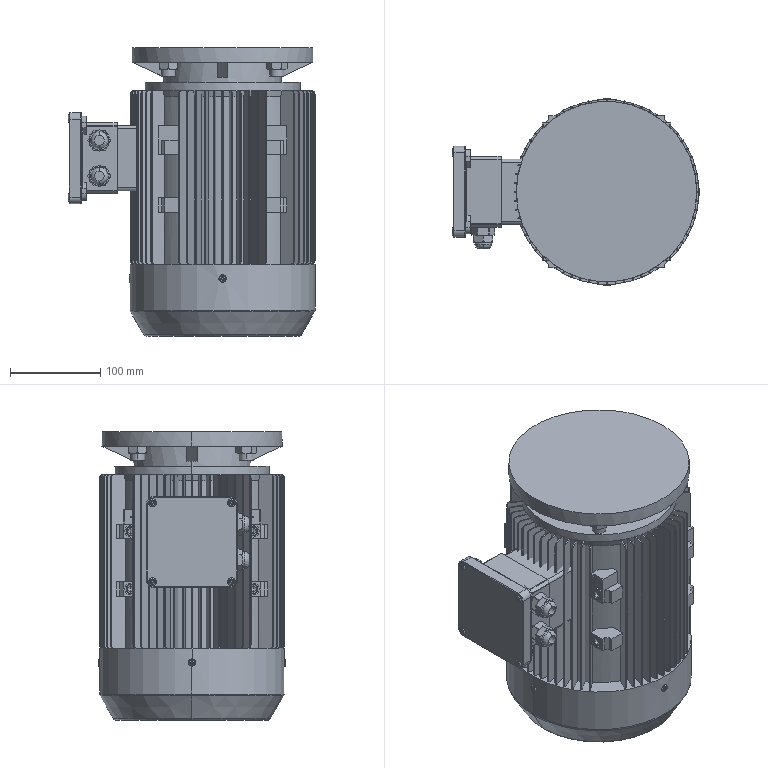Part | SolidWorks | features ICE 28, Fillet 9, MirrorPattern 5, CirPattern 4, DeleteBody 4, Chamfer 2, Revolution 2, Extrusion 1, MirrorSolid 1, RevCut 1, SketchPattern 1 | 2 solids | 1317 faces | box 274.826 x 207.05 x 320 mm | volume 8806469 mm3 | plane 776 | cylinder 372 | cone 121 | torus 48 | commonest cylinder face diameters 8.2 x112 168.1 x52 0.492 x32 0.52 x32 1.446 x28 1.968 x16